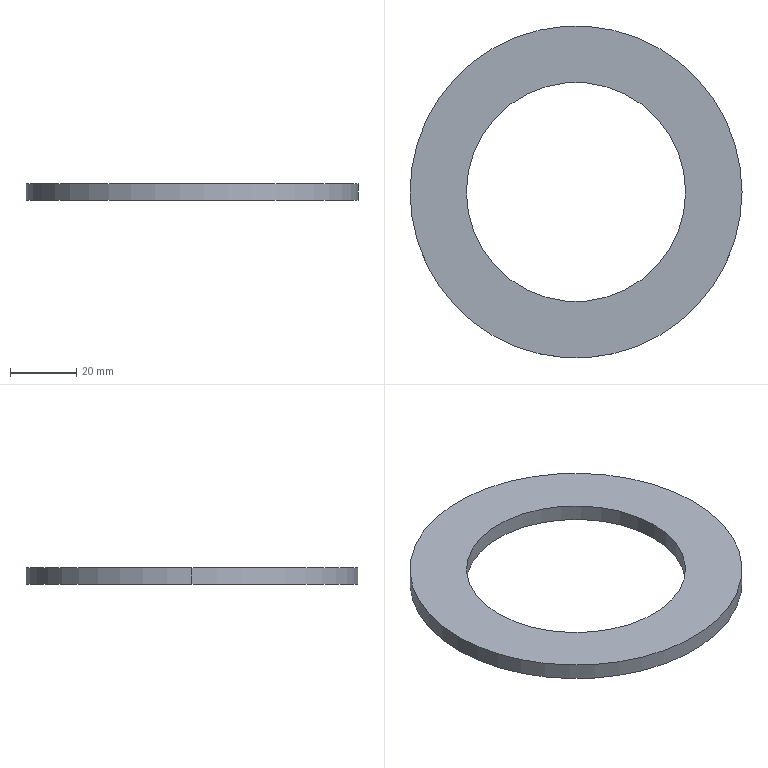Part | SolidWorks | features Extrusion 1 | 1 solid | 6 faces | box 100 x 100 x 5 mm | volume 22164 mm3 | cylinder 4 | plane 2 | commonest cylinder face diameters 66 x2 100 x2
STEP:
#1=CARTESIAN_POINT('',(-33.,0.,5.));
#2=VERTEX_POINT('',#1);
#3=CARTESIAN_POINT('',(33.,0.,5.));
#4=VERTEX_POINT('',#3);
#5=CARTESIAN_POINT('',(0.,0.,5.));
#6=DIRECTION('',(0.,0.,1.));
#7=DIRECTION('',(1.,0.,0.));
#8=AXIS2_PLACEMENT_3D('',#5,#6,#7);
#9=CIRCLE('',#8,33.);
#10=EDGE_CURVE('',#2,#4,#9,.T.);
#11=ORIENTED_EDGE('',*,*,#10,.T.);
#12=CARTESIAN_POINT('',(33.,0.,0.));
#13=VERTEX_POINT('',#12);
#14=CARTESIAN_POINT('',(33.,0.,5.));
#15=DIRECTION('',(0.,0.,-1.));
#16=VECTOR('',#15,1000.);
#17=LINE('',#14,#16);
#18=EDGE_CURVE('',#4,#13,#17,.T.);
#19=ORIENTED_EDGE('',*,*,#18,.T.);
#20=CARTESIAN_POINT('',(-33.,0.,0.));
#21=VERTEX_POINT('',#20);
#22=CARTESIAN_POINT('',(0.,0.,0.));
#23=DIRECTION('',(0.,0.,1.));
#24=DIRECTION('',(1.,0.,0.));
#25=AXIS2_PLACEMENT_3D('',#22,#23,#24);
#26=CIRCLE('',#25,33.);
#27=EDGE_CURVE('',#21,#13,#26,.T.);
#28=ORIENTED_EDGE('',*,*,#27,.F.);
#29=CARTESIAN_POINT('',(-33.,0.,5.));
#30=DIRECTION('',(0.,0.,-1.));
#31=VECTOR('',#30,1000.);
#32=LINE('',#29,#31);
#33=EDGE_CURVE('',#2,#21,#32,.T.);
#34=ORIENTED_EDGE('',*,*,#33,.F.);
#35=EDGE_LOOP('',(#11,#19,#28,#34));
#36=FACE_OUTER_BOUND('',#35,.T.);
#37=CARTESIAN_POINT('',(0.,0.,5.));
#38=DIRECTION('',(0.,0.,-1.));
#39=DIRECTION('',(-1.,0.,0.));
#40=AXIS2_PLACEMENT_3D('',#37,#38,#39);
#41=CYLINDRICAL_SURFACE('',#40,33.);
#42=ADVANCED_FACE('',(#36),#41,.F.);
#43=CARTESIAN_POINT('',(50.,0.,5.));
#44=VERTEX_POINT('',#43);
#45=CARTESIAN_POINT('',(-50.,0.,5.));
#46=VERTEX_POINT('',#45);
#47=CARTESIAN_POINT('',(0.,0.,5.));
#48=DIRECTION('',(0.,0.,1.));
#49=DIRECTION('',(1.,0.,0.));
#50=AXIS2_PLACEMENT_3D('',#47,#48,#49);
#51=CIRCLE('',#50,50.);
#52=EDGE_CURVE('',#44,#46,#51,.T.);
#53=ORIENTED_EDGE('',*,*,#52,.F.);
#54=CARTESIAN_POINT('',(50.,0.,0.));
#55=VERTEX_POINT('',#54);
#56=CARTESIAN_POINT('',(50.,0.,5.));
#57=DIRECTION('',(0.,0.,-1.));
#58=VECTOR('',#57,1000.);
#59=LINE('',#56,#58);
#60=EDGE_CURVE('',#44,#55,#59,.T.);
#61=ORIENTED_EDGE('',*,*,#60,.T.);
#62=CARTESIAN_POINT('',(-50.,0.,0.));
#63=VERTEX_POINT('',#62);
#64=CARTESIAN_POINT('',(0.,0.,0.));
#65=DIRECTION('',(0.,0.,1.));
#66=DIRECTION('',(1.,0.,0.));
#67=AXIS2_PLACEMENT_3D('',#64,#65,#66);
#68=CIRCLE('',#67,50.);
#69=EDGE_CURVE('',#55,#63,#68,.T.);
#70=ORIENTED_EDGE('',*,*,#69,.T.);
#71=CARTESIAN_POINT('',(-50.,0.,5.));
#72=DIRECTION('',(0.,0.,-1.));
#73=VECTOR('',#72,1000.);
#74=LINE('',#71,#73);
#75=EDGE_CURVE('',#46,#63,#74,.T.);
#76=ORIENTED_EDGE('',*,*,#75,.F.);
#77=EDGE_LOOP('',(#53,#61,#70,#76));
#78=FACE_OUTER_BOUND('',#77,.T.);
#79=CARTESIAN_POINT('',(0.,0.,5.));
#80=DIRECTION('',(0.,0.,-1.));
#81=DIRECTION('',(-1.,0.,0.));
#82=AXIS2_PLACEMENT_3D('',#79,#80,#81);
#83=CYLINDRICAL_SURFACE('',#82,50.);
#84=ADVANCED_FACE('',(#78),#83,.T.);
#85=CARTESIAN_POINT('',(0.,0.,5.));
#86=DIRECTION('',(0.,0.,1.));
#87=DIRECTION('',(1.,0.,0.));
#88=AXIS2_PLACEMENT_3D('',#85,#86,#87);
#89=CIRCLE('',#88,50.);
#90=EDGE_CURVE('',#46,#44,#89,.T.);
#91=ORIENTED_EDGE('',*,*,#90,.T.);
#92=ORIENTED_EDGE('',*,*,#52,.T.);
#93=EDGE_LOOP('',(#91,#92));
#94=FACE_OUTER_BOUND('',#93,.T.);
#95=ORIENTED_EDGE('',*,*,#10,.F.);
#96=CARTESIAN_POINT('',(0.,0.,5.));
#97=DIRECTION('',(0.,0.,1.));
#98=DIRECTION('',(1.,0.,0.));
#99=AXIS2_PLACEMENT_3D('',#96,#97,#98);
#100=CIRCLE('',#99,33.);
#101=EDGE_CURVE('',#4,#2,#100,.T.);
#102=ORIENTED_EDGE('',*,*,#101,.F.);
#103=EDGE_LOOP('',(#95,#102));
#104=FACE_BOUND('',#103,.T.);
#105=CARTESIAN_POINT('',(0.,0.,5.));
#106=DIRECTION('',(0.,0.,1.));
#107=DIRECTION('',(1.,0.,0.));
#108=AXIS2_PLACEMENT_3D('',#105,#106,#107);
#109=PLANE('',#108);
#110=ADVANCED_FACE('',(#94,#104),#109,.T.);
#111=CARTESIAN_POINT('',(0.,0.,0.));
#112=DIRECTION('',(0.,0.,1.));
#113=DIRECTION('',(1.,0.,0.));
#114=AXIS2_PLACEMENT_3D('',#111,#112,#113);
#115=CIRCLE('',#114,50.);
#116=EDGE_CURVE('',#63,#55,#115,.T.);
#117=ORIENTED_EDGE('',*,*,#116,.F.);
#118=ORIENTED_EDGE('',*,*,#69,.F.);
#119=EDGE_LOOP('',(#117,#118));
#120=FACE_OUTER_BOUND('',#119,.T.);
#121=ORIENTED_EDGE('',*,*,#27,.T.);
#122=CARTESIAN_POINT('',(0.,0.,0.));
#123=DIRECTION('',(0.,0.,1.));
#124=DIRECTION('',(1.,0.,0.));
#125=AXIS2_PLACEMENT_3D('',#122,#123,#124);
#126=CIRCLE('',#125,33.);
#127=EDGE_CURVE('',#13,#21,#126,.T.);
#128=ORIENTED_EDGE('',*,*,#127,.T.);
#129=EDGE_LOOP('',(#121,#128));
#130=FACE_BOUND('',#129,.T.);
#131=CARTESIAN_POINT('',(0.,0.,0.));
#132=DIRECTION('',(0.,0.,1.));
#133=DIRECTION('',(1.,0.,0.));
#134=AXIS2_PLACEMENT_3D('',#131,#132,#133);
#135=PLANE('',#134);
#136=ADVANCED_FACE('',(#120,#130),#135,.F.);
#137=ORIENTED_EDGE('',*,*,#60,.F.);
#138=ORIENTED_EDGE('',*,*,#90,.F.);
#139=ORIENTED_EDGE('',*,*,#75,.T.);
#140=ORIENTED_EDGE('',*,*,#116,.T.);
#141=EDGE_LOOP('',(#137,#138,#139,#140));
#142=FACE_OUTER_BOUND('',#141,.T.);
#143=CARTESIAN_POINT('',(0.,0.,5.));
#144=DIRECTION('',(0.,0.,-1.));
#145=DIRECTION('',(-1.,0.,0.));
#146=AXIS2_PLACEMENT_3D('',#143,#144,#145);
#147=CYLINDRICAL_SURFACE('',#146,50.);
#148=ADVANCED_FACE('',(#142),#147,.T.);
#149=ORIENTED_EDGE('',*,*,#18,.F.);
#150=ORIENTED_EDGE('',*,*,#101,.T.);
#151=ORIENTED_EDGE('',*,*,#33,.T.);
#152=ORIENTED_EDGE('',*,*,#127,.F.);
#153=EDGE_LOOP('',(#149,#150,#151,#152));
#154=FACE_OUTER_BOUND('',#153,.T.);
#155=CARTESIAN_POINT('',(0.,0.,5.));
#156=DIRECTION('',(0.,0.,-1.));
#157=DIRECTION('',(-1.,0.,0.));
#158=AXIS2_PLACEMENT_3D('',#155,#156,#157);
#159=CYLINDRICAL_SURFACE('',#158,33.);
#160=ADVANCED_FACE('',(#154),#159,.F.);
#161=CLOSED_SHELL('',(#42,#84,#110,#136,#148,#160));
#162=MANIFOLD_SOLID_BREP('',#161);
#163=CARTESIAN_POINT('',(0.,0.,0.));
#164=DIRECTION('',(0.,0.,1.));
#165=DIRECTION('',(1.,0.,0.));
#166=AXIS2_PLACEMENT_3D('',#163,#164,#165);
#167=(LENGTH_UNIT()NAMED_UNIT(*)SI_UNIT(.MILLI.,.METRE.));
#168=UNCERTAINTY_MEASURE_WITH_UNIT(LENGTH_MEASURE(0.00001),#167,'','');
#169=(NAMED_UNIT(*)PLANE_ANGLE_UNIT()SI_UNIT($,.RADIAN.));
#170=(NAMED_UNIT(*)SI_UNIT($,.STERADIAN.)SOLID_ANGLE_UNIT());
#171=(GEOMETRIC_REPRESENTATION_CONTEXT(3)GLOBAL_UNCERTAINTY_ASSIGNED_CONTEXT((#168))GLOBAL_UNIT_ASSIGNED_CONTEXT((#167,#169,#170))REPRESENTATION_CONTEXT('',''));
#172=ADVANCED_BREP_SHAPE_REPRESENTATION('',(#162,#166),#171);